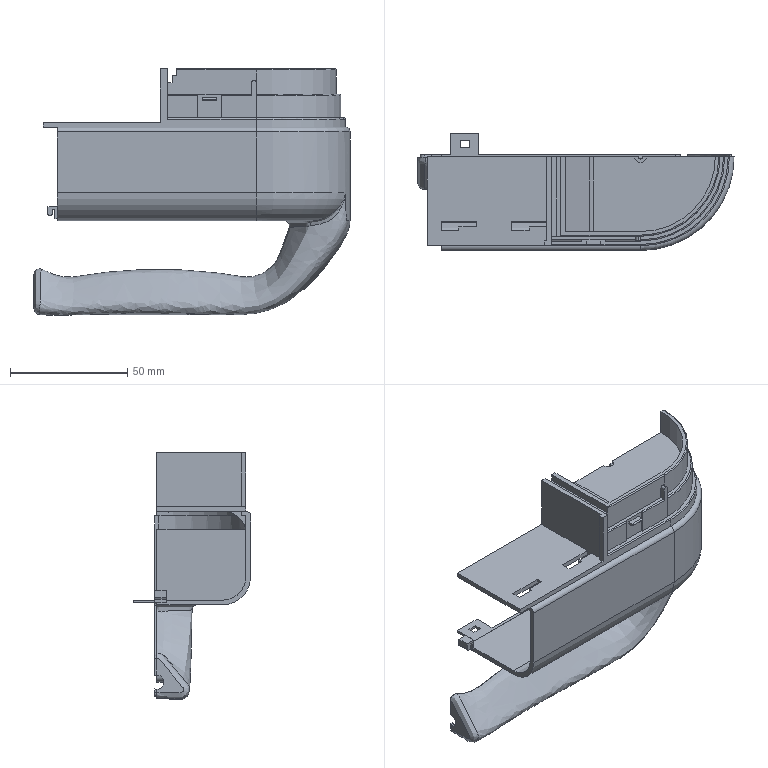Part | SolidWorks | features ICE 11, Fillet 1, LPattern 1, Rib 1, Stock 1 | 1 solid | 221 faces | box 135 x 50.019 x 105.415 mm | volume 49896 mm3 | plane 144 | cylinder 53 | spline 18 | torus 6 | commonest cylinder face diameters 6 x11 1 x10 3 x8 20 x4 2 x3 4 x2